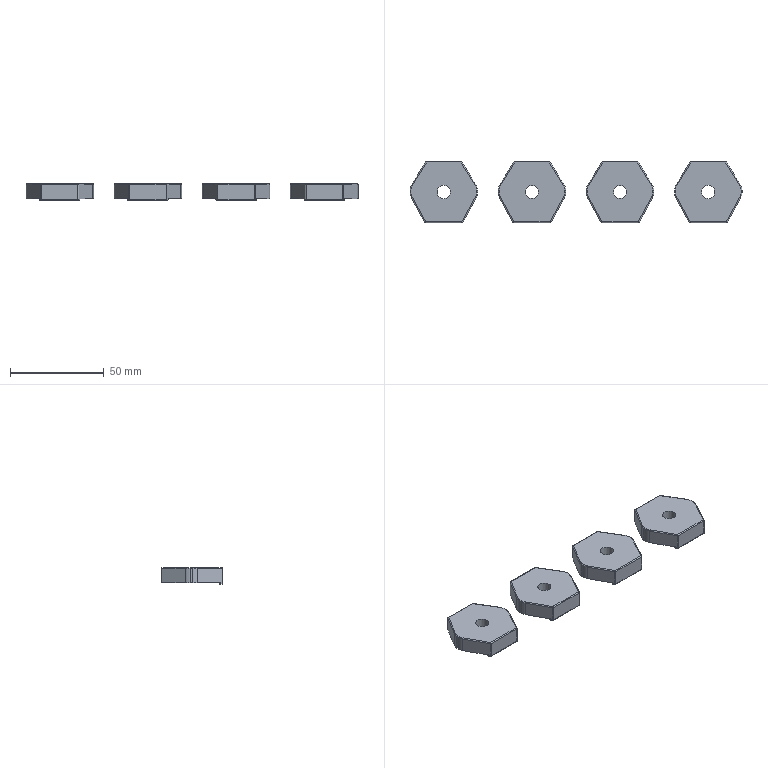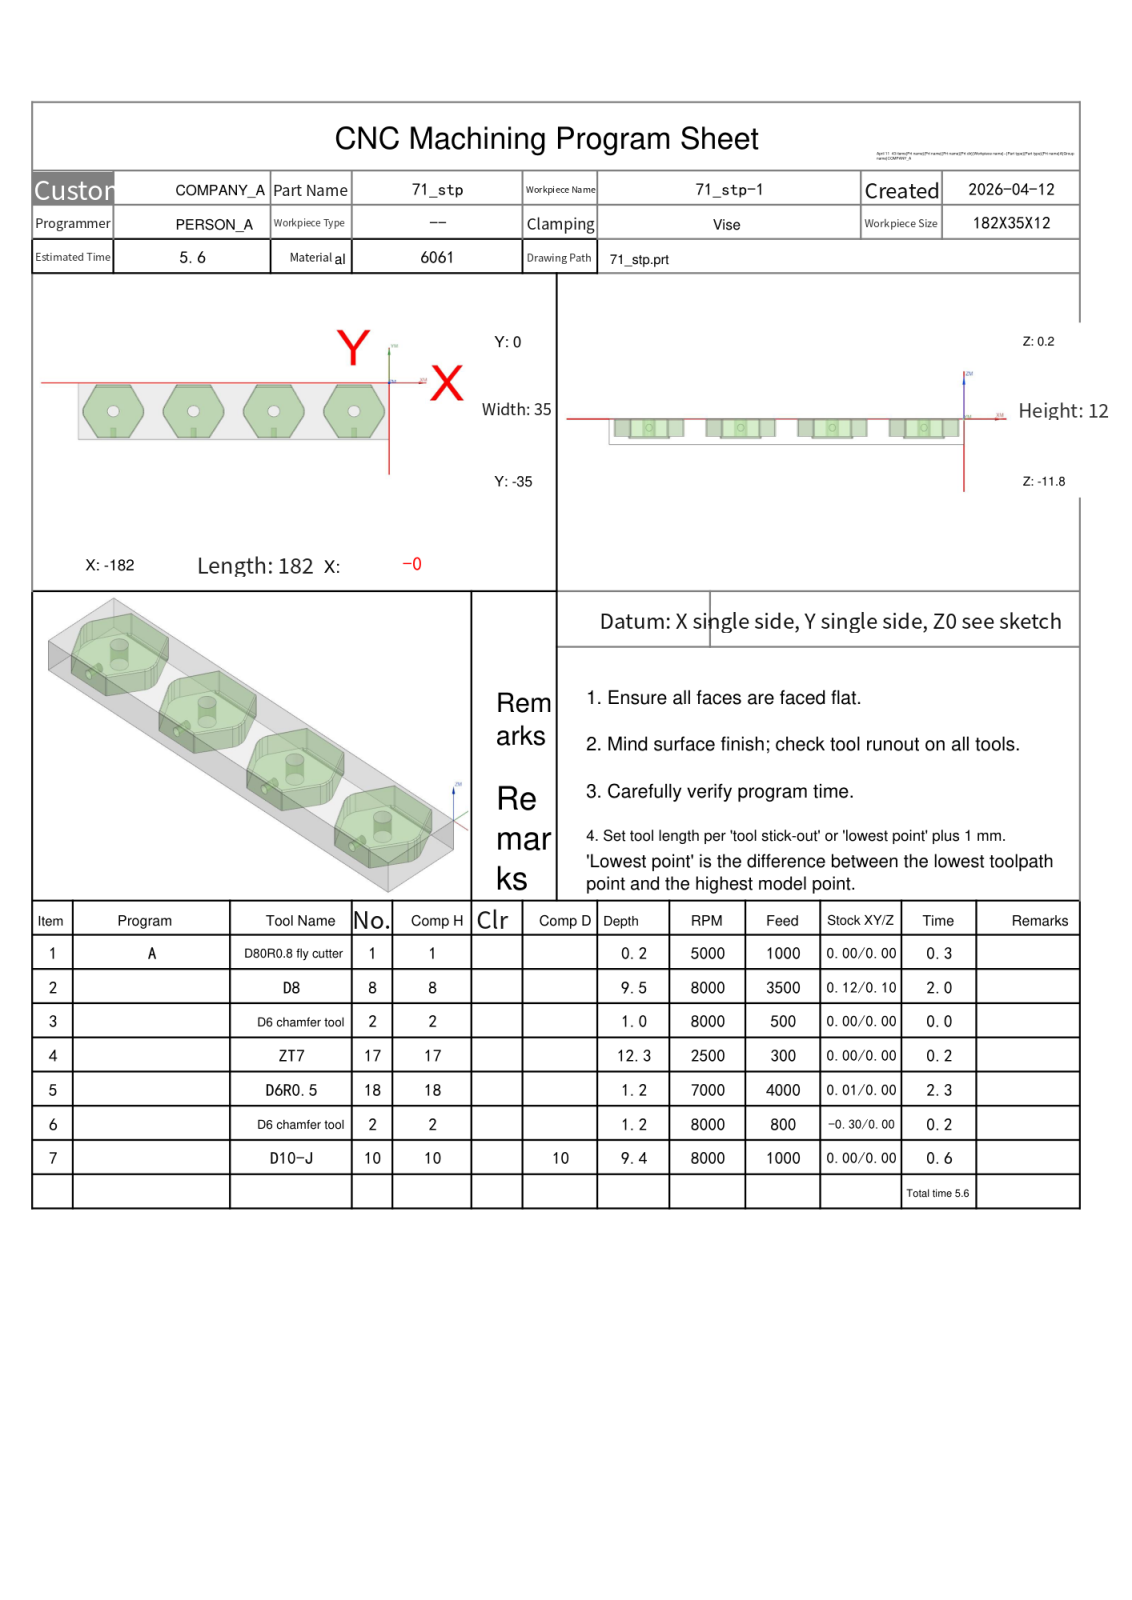NC program | NX | posted by the shop | part box 177 x 33 x 9 mm
Lines 3114 to 4443 of 15773:
N5 T18 M06
(D6R0.5  D=6. R=0.5 H=18 ce=0.01 di=0.00)
(MAX_Z=20. MIN_Z=-1. Time=2.28M)
G00 G90 G54 X-38.65 Y-23.77 M03 S7000
G43 H18 Z20.
M08
Z1.5
G01 X-39.759 Y-21.951 Z1.388 F4000.
X-40.062 Y-21.345 Z1.353
X-40.306 Y-20.712 Z1.317
X-40.489 Y-20.059 Z1.282
X-40.61 Y-19.392 Z1.246
X-40.668 Y-18.716 Z1.211
Y-16.764 Z1.108
X-40.599 Y-16.011 Z1.069
X-40.453 Y-15.269 Z1.029
X-40.228 Y-14.547 Z.989
X-39.929 Y-13.852 Z.95
X-32.47 Y-.086 Z.129
X-32.218 Y.255 Z.107
X-31.915 Y.551 Z.085
X-31.57 Y.796 Z.063
X-31.19 Y.983 Z.04
X-30.785 Y1.108 Z.018
X-30.366 Y1.168 Z-.004
X-30.202 Z-.012
X-10.798
G02 X-8.452 Y-.229 I0.0 J-2.668
G01 X-1.198 Y-13.617
G02 X-.332 Y-17.032 I-6.302 J-3.415
G01 Y-18.448
G02 X-1.38 Y-22.18 I-7.168 J0.0
G01 X-9.13 Y-34.889
G02 X-11.408 Y-36.168 I-2.277 J1.389
G01 X-29.592
G02 X-31.87 Y-34.889 I0.0 J2.668
G01 X-39.62 Y-22.18
G02 X-40.668 Y-18.448 I6.12 J3.732
G01 Y-17.032
G02 X-39.802 Y-13.617 I7.168 J0.0
G01 X-32.548 Y-.229
G02 X-30.202 Y1.168 I2.345 J-1.271
G01 X-27.777 Y1.169 Z-.013
X-25.351 Y1.172
X-22.926 Y1.175 Z-.014
X-20.5 Y1.177
X-18.074 Y1.18 Z-.015
X-15.649 Y1.182
X-13.223 Y1.184
X-10.798 Y1.187 Z-.016
X-10.637 Y1.182
X-10.478 Y1.168
X-10.319 Y1.144
X-10.162 Y1.111
X-10.008 Y1.069
X-9.856 Y1.017
X-9.707 Y.957
X-9.563 Y.887
X-9.422 Y.81
X-9.287 Y.724
X-9.157 Y.63
X-9.033 Y.528
X-8.915 Y.419
X-8.804 Y.304
X-8.699 Y.182
X-8.603 Y.054
X-8.514 Y-.08
X-8.433 Y-.219
X-7.222 Y-2.449 Z-.017
X-6.011 Y-4.679
X-4.799 Y-6.909 Z-.018
X-3.589 Y-9.14
X-2.377 Y-11.369 Z-.019
X-1.167 Y-13.6
X-1.106 Y-13.713
X-1.049 Y-13.826
X-.993 Y-13.941
X-.939 Y-14.057
X-.887 Y-14.174
X-.837 Y-14.292
X-.79 Y-14.41
X-.745 Y-14.53
X-.701 Y-14.65
X-.659 Y-14.771
X-.62 Y-14.892
X-.584 Y-15.015
X-.548 Y-15.137
X-.516 Y-15.261
X-.485 Y-15.385
X-.458 Y-15.51
X-.431 Y-15.635
X-.407 Y-15.76
X-.386 Y-15.886
X-.367 Y-16.013
X-.35 Y-16.139
X-.335 Y-16.266
X-.322 Y-16.393
X-.312 Y-16.521 Z-.02
X-.298 Y-16.776
X-.294 Y-17.032
X-.292 Y-17.74
X-.293 Y-18.448
X-.296 Y-18.695
X-.309 Y-18.941
X-.329 Y-19.187
X-.359 Y-19.432
X-.396 Y-19.676
X-.443 Y-19.918
X-.497 Y-20.159
X-.559 Y-20.398
X-.63 Y-20.634
X-.708 Y-20.868
X-.795 Y-21.099
X-.889 Y-21.327
X-.991 Y-21.552
X-1.101 Y-21.773
X-1.218 Y-21.99
X-1.343 Y-22.203 Z-.021
X-2.633 Y-24.322
X-3.923 Y-26.441
X-5.213 Y-28.561 Z-.022
X-6.502 Y-30.68
X-7.793 Y-32.798 Z-.023
X-9.082 Y-34.918
X-9.167 Y-35.048
X-9.258 Y-35.173
X-9.356 Y-35.292
X-9.462 Y-35.406
X-9.573 Y-35.513
X-9.69 Y-35.614
X-9.813 Y-35.709
X-9.941 Y-35.796
X-10.074 Y-35.876
X-10.211 Y-35.948
X-10.352 Y-36.012
X-10.496 Y-36.068
X-10.643 Y-36.116
X-10.793 Y-36.155
X-10.945 Y-36.186 Z-.024
X-11.098 Y-36.208
X-11.253 Y-36.221
X-11.408 Y-36.225
X-13.681 Y-36.226
X-15.954 Y-36.229
X-18.227 Y-36.23 Z-.025
X-20.5 Y-36.232
X-22.773 Y-36.234 Z-.026
X-25.046 Y-36.236
X-27.319 Y-36.237
X-29.592 Y-36.239 Z-.027
X-29.748 Y-36.235
X-29.903 Y-36.221
X-30.057 Y-36.2
X-30.21 Y-36.169
X-30.361 Y-36.13
X-30.509 Y-36.082
X-30.654 Y-36.026
X-30.796 Y-35.961
X-30.934 Y-35.889
X-31.067 Y-35.809
X-31.197 Y-35.722
X-31.32 Y-35.627
X-31.438 Y-35.526
X-31.55 Y-35.418
X-31.657 Y-35.303
X-31.755 Y-35.183
X-31.848 Y-35.058
X-31.933 Y-34.927
X-33.226 Y-32.81 Z-.028
X-34.519 Y-30.693
X-35.813 Y-28.576 Z-.029
X-37.105 Y-26.458
X-38.399 Y-24.341
X-39.692 Y-22.224 Z-.03
X-39.817 Y-22.01
X-39.936 Y-21.792
X-40.046 Y-21.57
X-40.15 Y-21.344
X-40.245 Y-21.115
X-40.332 Y-20.883
X-40.412 Y-20.647
X-40.483 Y-20.41
X-40.546 Y-20.17
X-40.601 Y-19.928
X-40.648 Y-19.684
X-40.686 Y-19.438
X-40.716 Y-19.192
X-40.738 Y-18.945
X-40.75 Y-18.697
X-40.755 Y-18.448
X-40.756 Y-17.74 Z-.031
Y-17.032
X-40.751 Y-16.774
X-40.738 Y-16.517
X-40.715 Y-16.261
X-40.684 Y-16.006
X-40.643 Y-15.751
X-40.593 Y-15.499
X-40.534 Y-15.248
X-40.467 Y-15.
X-40.391 Y-14.754
X-40.306 Y-14.511
X-40.212 Y-14.271
X-40.11 Y-14.035
X-40. Y-13.802
X-39.882 Y-13.574
X-38.674 Y-11.342 Z-.032
X-37.466 Y-9.11
X-36.259 Y-6.877 Z-.033
X-35.051 Y-4.645
X-33.843 Y-2.414 Z-.034
X-32.636 Y-.181
X-32.596 Y-.109
X-32.553 Y-.038
X-32.509 Y.031
X-32.462 Y.099
X-32.413 Y.166
X-32.363 Y.231
X-32.31 Y.295
X-32.255 Y.357
X-32.199 Y.418
X-32.141 Y.476
X-32.081 Y.533
X-32.02 Y.588
X-31.957 Y.642
X-31.892 Y.693
X-31.826 Y.743
X-31.758 Y.79
X-31.689 Y.836
X-31.619 Y.879
X-31.548 Y.92
X-31.475 Y.959
X-31.401 Y.997
X-31.326 Y1.031
X-31.25 Y1.064
X-31.173 Y1.093
X-31.095 Y1.122
X-31.016 Y1.147
X-30.937 Y1.17
X-30.857 Y1.191
X-30.777 Y1.21
X-30.695 Y1.225
X-30.614 Y1.239
X-30.532 Y1.25
X-30.367 Y1.265
X-30.202 Y1.27 Z-.035
X-27.777 Y1.272
X-25.351 Y1.274 Z-.036
X-22.926 Y1.276
X-20.5 Y1.279 Z-.037
X-18.074 Y1.28 Z-.038
X-15.649 Y1.283
X-13.223 Y1.285 Z-.039
X-10.798 Y1.287
X-10.715 Y1.286
X-10.632 Y1.283
X-10.549 Y1.277
X-10.466 Y1.268
X-10.383 Y1.257
X-10.301 Y1.243
X-10.22 Y1.227
X-10.139 Y1.209
X-10.058 Y1.188 Z-.04
X-9.978 Y1.165
X-9.899 Y1.139
X-9.821 Y1.111
X-9.743 Y1.081
X-9.667 Y1.049
X-9.591 Y1.014
X-9.516 Y.977
X-9.443 Y.938
X-9.371 Y.896
X-9.3 Y.853
X-9.231 Y.807
X-9.162 Y.759
X-9.096 Y.709
X-9.03 Y.658
X-8.967 Y.604
X-8.905 Y.549
X-8.845 Y.491
X-8.786 Y.432
X-8.729 Y.371
X-8.674 Y.309
X-8.621 Y.244
X-8.57 Y.179
X-8.521 Y.112
X-8.473 Y.043
X-8.429 Y-.027
X-8.385 Y-.098
X-8.345 Y-.171
X-7.134 Y-2.401 Z-.041
X-5.923 Y-4.632
X-4.712 Y-6.862 Z-.042
X-3.501 Y-9.092 Z-.043
X-2.29 Y-11.322
X-1.08 Y-13.553 Z-.044
X-.96 Y-13.782
X-.849 Y-14.016
X-.746 Y-14.254
X-.652 Y-14.495
X-.565 Y-14.74
X-.489 Y-14.987
X-.42 Y-15.237
X-.361 Y-15.489
X-.31 Y-15.743
X-.269 Y-15.999
X-.236 Y-16.256 Z-.045
X-.214 Y-16.514
X-.199 Y-16.773
X-.194 Y-17.032
Y-17.74
Y-18.448
X-.197 Y-18.699
X-.21 Y-18.948
X-.231 Y-19.197
X-.261 Y-19.446
X-.299 Y-19.693
X-.346 Y-19.939
X-.401 Y-20.183 Z-.046
X-.464 Y-20.424
X-.535 Y-20.664
X-.615 Y-20.901
X-.703 Y-21.135
X-.799 Y-21.366
X-.902 Y-21.594
X-1.014 Y-21.818
X-1.133 Y-22.038
X-1.259 Y-22.254
X-2.549 Y-24.373 Z-.047
X-3.839 Y-26.492
X-5.129 Y-28.612 Z-.048
X-6.419 Y-30.731 Z-.049
X-7.709 Y-32.85
X-8.999 Y-34.969 Z-.05
X-9.086 Y-35.103
X-9.181 Y-35.233
X-9.283 Y-35.357
X-9.391 Y-35.474
X-9.507 Y-35.586
X-9.628 Y-35.691
X-9.756 Y-35.788
X-9.888 Y-35.879
X-10.026 Y-35.961
X-10.168 Y-36.036
X-10.314 Y-36.102
X-10.463 Y-36.16
X-10.616 Y-36.21
X-10.771 Y-36.25
X-10.928 Y-36.282
X-11.087 Y-36.305
X-11.247 Y-36.319
X-11.408 Y-36.323
X-13.681 Y-36.325 Z-.051
X-15.954 Y-36.327 Z-.052
X-18.227 Y-36.328
X-20.5 Y-36.33 Z-.053
X-22.773 Y-36.331
X-25.046 Y-36.333 Z-.054
X-27.319 Y-36.335
X-29.592 Y-36.337 Z-.055
X-29.754 Y-36.332
X-29.914 Y-36.318
X-30.074 Y-36.296
X-30.232 Y-36.264
X-30.388 Y-36.224
X-30.542 Y-36.174
X-30.692 Y-36.116
X-30.839 Y-36.049
X-30.982 Y-35.974
X-31.12 Y-35.891
X-31.254 Y-35.801
X-31.382 Y-35.703
X-31.504 Y-35.598 Z-.056
X-31.62 Y-35.486
X-31.73 Y-35.368
X-31.833 Y-35.243
X-31.928 Y-35.113
X-32.016 Y-34.978
X-33.309 Y-32.861
X-34.602 Y-30.743 Z-.057
X-35.895 Y-28.626 Z-.058
X-37.188 Y-26.509
X-38.481 Y-24.392 Z-.059
X-39.775 Y-22.275
X-39.902 Y-22.058
X-40.022 Y-21.837 Z-.06
X-40.134 Y-21.612
X-40.239 Y-21.383
X-40.336 Y-21.151
X-40.424 Y-20.915
X-40.505 Y-20.677
X-40.577 Y-20.436
X-40.641 Y-20.193
X-40.697 Y-19.947
X-40.744 Y-19.7
X-40.783 Y-19.452
X-40.813 Y-19.202
X-40.835 Y-18.951
X-40.848 Y-18.7
X-40.852 Y-18.448
Y-17.74 Z-.061
X-40.853 Y-17.032
X-40.849 Y-16.771
X-40.835 Y-16.51
X-40.812 Y-16.251
X-40.78 Y-15.992
X-40.739 Y-15.734
X-40.688 Y-15.478
X-40.629 Y-15.224
X-40.561 Y-14.973
X-40.483 Y-14.723
X-40.397 Y-14.477
X-40.302 Y-14.234
X-40.199 Y-13.995 Z-.062
X-40.087 Y-13.759
X-39.967 Y-13.527
X-38.76 Y-11.295
X-37.552 Y-9.063 Z-.063
X-36.345 Y-6.831 Z-.064
X-35.137 Y-4.599
X-33.929 Y-2.367 Z-.065
X-32.722 Y-.135
X-32.68 Y-.06
X-32.636 Y.013 Z-.066
X-32.59 Y.085
X-32.541 Y.156
X-32.491 Y.225
X-32.438 Y.292
X-32.384 Y.358
X-32.328 Y.422
X-32.27 Y.485
X-32.209 Y.546
X-32.148 Y.605
X-32.084 Y.662
X-32.019 Y.717
X-31.952 Y.77
X-31.883 Y.822
X-31.813 Y.871
X-31.742 Y.918
X-31.669 Y.963
X-31.595 Y1.006
X-31.519 Y1.046
X-31.443 Y1.085
X-31.365 Y1.12
X-31.287 Y1.154
X-31.207 Y1.185
X-31.127 Y1.214
X-31.045 Y1.24
X-30.963 Y1.264
X-30.88 Y1.286
X-30.797 Y1.305
X-30.713 Y1.321
X-30.628 Y1.336
X-30.544 Y1.347
X-30.459 Y1.356
X-30.373 Y1.362
X-30.288 Y1.366
X-30.202 Y1.368
X-27.777 Y1.369 Z-.067
X-25.351 Y1.372 Z-.068
X-22.926 Y1.373 Z-.069
X-20.5 Y1.376
X-18.074 Y1.377 Z-.07
X-15.649 Y1.38 Z-.071
X-13.223 Y1.381 Z-.072
X-10.798 Y1.383
X-10.643 Y1.379
X-10.489 Y1.367 Z-.073
X-10.335 Y1.346
X-10.183 Y1.318
X-10.033 Y1.281
X-9.884 Y1.236
X-9.739 Y1.183
X-9.596 Y1.122
X-9.457 Y1.054
X-9.322 Y.978
X-9.191 Y.896
X-9.064 Y.806
X-8.943 Y.71
X-8.827 Y.607
X-8.717 Y.498
X-8.612 Y.384
X-8.514 Y.264
X-8.423 Y.139
X-8.338 Y.009
X-8.261 Y-.125
X-7.05 Y-2.356 Z-.074
X-5.839 Y-4.586 Z-.075
X-4.629 Y-6.817 Z-.076
X-3.418 Y-9.047 Z-.077
X-2.207 Y-11.277
X-.996 Y-13.507 Z-.078
X-.875 Y-13.74
X-.762 Y-13.977
X-.658 Y-14.218 Z-.079
X-.562 Y-14.462
X-.475 Y-14.71
X-.397 Y-14.96
X-.328 Y-15.213
X-.268 Y-15.469
X-.217 Y-15.726
X-.175 Y-15.985
X-.142 Y-16.246
X-.119 Y-16.507
X-.104 Y-16.769
X-.1 Y-17.032
X-.099 Y-17.74 Z-.08
Y-18.448
X-.103 Y-18.702
X-.116 Y-18.955
X-.137 Y-19.207
X-.167 Y-19.459
X-.206 Y-19.709
X-.253 Y-19.958
X-.309 Y-20.205
X-.373 Y-20.45 Z-.081
X-.445 Y-20.693
X-.526 Y-20.933
X-.615 Y-21.17
X-.712 Y-21.404
X-.817 Y-21.635
X-.93 Y-21.862
X-1.05 Y-22.085
X-1.178 Y-22.303
X-2.469 Y-24.422 Z-.082
X-3.758 Y-26.542 Z-.083
X-5.049 Y-28.66 Z-.084
X-6.338 Y-30.78
X-7.629 Y-32.899 Z-.085
X-8.918 Y-35.018 Z-.086
X-9.009 Y-35.157
X-9.106 Y-35.291
X-9.212 Y-35.418
X-9.324 Y-35.54
X-9.444 Y-35.655
X-9.569 Y-35.764
X-9.701 Y-35.864
X-9.838 Y-35.958
X-9.98 Y-36.043
X-10.126 Y-36.12
X-10.277 Y-36.189 Z-.087
X-10.432 Y-36.249
X-10.59 Y-36.3
X-10.75 Y-36.342
X-10.912 Y-36.375
X-11.077 Y-36.399
X-11.242 Y-36.413
X-11.408 Y-36.418
X-13.681 Y-36.419 Z-.088
X-15.954 Y-36.421
X-18.227 Y-36.422 Z-.089
X-20.5 Y-36.424 Z-.09
X-22.773 Y-36.426 Z-.091
X-25.046 Y-36.427
X-27.319 Y-36.429 Z-.092
X-29.592 Y-36.43 Z-.093
X-29.759 Y-36.426
X-29.925 Y-36.411
X-30.09 Y-36.388
X-30.253 Y-36.355
X-30.414 Y-36.313
X-30.573 Y-36.262
X-30.728 Y-36.202
X-30.88 Y-36.133
X-31.028 Y-36.056
X-31.17 Y-35.97
X-31.308 Y-35.877
X-31.441 Y-35.775
X-31.567 Y-35.667
X-31.687 Y-35.551
X-31.8 Y-35.429 Z-.094
X-31.906 Y-35.301
X-32.005 Y-35.166
X-32.096 Y-35.027
X-33.389 Y-32.909
X-34.682 Y-30.792 Z-.095
X-35.975 Y-28.675 Z-.096
X-37.268 Y-26.558 Z-.097
X-38.561 Y-24.44 Z-.098
X-39.854 Y-22.323
X-39.983 Y-22.104 Z-.099
X-40.105 Y-21.88
X-40.218 Y-21.652
X-40.324 Y-21.42
X-40.422 Y-21.185
X-40.512 Y-20.946
X-40.593 Y-20.705
X-40.666 Y-20.461
X-40.731 Y-20.215
X-40.788 Y-19.966
X-40.836 Y-19.716
X-40.875 Y-19.464
X-40.905 Y-19.212
X-40.927 Y-18.958 Z-.1
X-40.941 Y-18.703
X-40.945 Y-18.448
X-40.946 Y-17.74
Y-17.032
X-40.942 Y-16.768
X-40.928 Y-16.504
X-40.904 Y-16.241
X-40.872 Y-15.979 Z-.101
X-40.83 Y-15.718
X-40.779 Y-15.459
X-40.719 Y-15.201
X-40.65 Y-14.947
X-40.571 Y-14.694
X-40.484 Y-14.445
X-40.388 Y-14.199
X-40.284 Y-13.956
X-40.17 Y-13.718
X-40.049 Y-13.483
X-38.841 Y-11.251 Z-.102
X-37.634 Y-9.019 Z-.103
X-36.426 Y-6.787 Z-.104
X-35.219 Y-4.555 Z-.105
X-34.011 Y-2.323
X-32.803 Y-.091 Z-.106
X-32.724 Y.047
X-32.637 Y.18
X-32.544 Y.309
X-32.443 Y.432
X-32.336 Y.549
X-32.223 Y.661 Z-.107
X-32.105 Y.767
X-31.98 Y.865
X-31.851 Y.958
X-31.716 Y1.043
X-31.578 Y1.12
X-31.435 Y1.19
X-31.289 Y1.253
X-31.14 Y1.307
X-30.988 Y1.354
X-30.833 Y1.392
X-30.677 Y1.422
X-30.52 Y1.443
X-30.361 Y1.456
X-30.202 Y1.461
X-27.777 Y1.462 Z-.108
X-25.351 Y1.464 Z-.109
X-22.926 Y1.465 Z-.11
X-20.5 Y1.468 Z-.111
X-18.074 Y1.469 Z-.112
X-15.649 Y1.471 Z-.113
X-13.223 Y1.473 Z-.114
X-10.798 Y1.475 Z-.115
X-10.638 Y1.471
X-10.479 Y1.458
X-10.32 Y1.437
X-10.163 Y1.407
X-10.008 Y1.369
X-9.855 Y1.322
X-9.705 Y1.268
X-9.558 Y1.205
X-9.415 Y1.135
X-9.275 Y1.057
X-9.14 Y.972
X-9.01 Y.879
X-8.884 Y.78 Z-.116
X-8.765 Y.674
X-8.651 Y.562
X-8.543 Y.443
X-8.442 Y.32
X-8.348 Y.191
X-8.26 Y.057
X-8.18 Y-.082
X-6.97 Y-2.312 Z-.117
X-5.759 Y-4.543 Z-.118
X-4.548 Y-6.773 Z-.119
X-3.338 Y-9.003 Z-.12
X-2.127 Y-11.234 Z-.121
X-.916 Y-13.464 Z-.122
X-.794 Y-13.7
X-.68 Y-13.94
X-.574 Y-14.183
X-.477 Y-14.431
X-.389 Y-14.681
X-.31 Y-14.935 Z-.123
X-.24 Y-15.191
X-.179 Y-15.45
X-.128 Y-15.71
X-.085 Y-15.973
X-.052 Y-16.236
X-.029 Y-16.501
X-.014 Y-16.766
X-.009 Y-17.032
Y-17.74 Z-.124
X-.008 Y-18.448
X-.012 Y-18.705
X-.025 Y-18.961
X-.047 Y-19.216
X-.078 Y-19.471
X-.117 Y-19.724
X-.165 Y-19.976
X-.221 Y-20.227 Z-.125
X-.286 Y-20.475
X-.359 Y-20.72
X-.441 Y-20.963
X-.531 Y-21.204
X-.629 Y-21.44
X-.735 Y-21.674
X-.85 Y-21.903
X-.971 Y-22.129
X-1.101 Y-22.351
X-2.391 Y-24.469 Z-.126
X-3.681 Y-26.588 Z-.127
X-4.972 Y-28.707 Z-.128
X-6.262 Y-30.827 Z-.129
X-7.552 Y-32.945 Z-.13
X-8.842 Y-35.065 Z-.131
X-8.935 Y-35.208
X-9.036 Y-35.346
X-9.144 Y-35.477
X-9.26 Y-35.603
X-9.383 Y-35.722 Z-.132
X-9.512 Y-35.833
X-9.648 Y-35.937
X-9.789 Y-36.033
X-9.936 Y-36.121
X-10.087 Y-36.201
X-10.243 Y-36.271
X-10.402 Y-36.333
X-10.564 Y-36.386
X-10.73 Y-36.429
X-10.897 Y-36.463
X-11.066 Y-36.488
X-11.237 Y-36.502
X-11.408 Y-36.507
X-13.681 Y-36.508 Z-.133
X-15.954 Y-36.51 Z-.134
X-18.227 Y-36.511 Z-.135
X-20.5 Y-36.513 Z-.136
X-22.773 Y-36.514 Z-.137
X-25.046 Y-36.516 Z-.138
X-27.319 Y-36.518 Z-.139
X-29.592 Y-36.519
X-29.678 Y-36.518
X-29.764 Y-36.514 Z-.14
X-29.85 Y-36.508
X-29.935 Y-36.5
X-30.02 Y-36.489
X-30.105 Y-36.476
X-30.189 Y-36.46
X-30.273 Y-36.442
X-30.357 Y-36.421
X-30.439 Y-36.399
X-30.521 Y-36.373
X-30.603 Y-36.346
X-30.683 Y-36.316
X-30.763 Y-36.284
X-30.841 Y-36.25
X-30.919 Y-36.213
X-30.996 Y-36.174
X-31.071 Y-36.133
X-31.145 Y-36.09
X-31.218 Y-36.045
X-31.29 Y-35.998
X-31.36 Y-35.949
X-31.429 Y-35.898
X-31.497 Y-35.844
X-31.563 Y-35.79
X-31.627 Y-35.733
X-31.69 Y-35.674
X-31.75 Y-35.613
X-31.81 Y-35.551
X-31.867 Y-35.488
X-31.923 Y-35.422
X-31.976 Y-35.355 Z-.141
X-32.028 Y-35.287
X-32.078 Y-35.217
X-32.126 Y-35.146
X-32.172 Y-35.073
X-33.465 Y-32.955 Z-.142
X-34.758 Y-30.838 Z-.143
X-36.05 Y-28.721 Z-.144
X-37.344 Y-26.604
X-38.636 Y-24.486 Z-.145
X-39.93 Y-22.369 Z-.146
X-40.06 Y-22.147 Z-.147
X-40.183 Y-21.92
X-40.298 Y-21.69
X-40.405 Y-21.455
X-40.504 Y-21.217
X-40.595 Y-20.976
X-40.677 Y-20.732
X-40.751 Y-20.485
X-40.817 Y-20.236
X-40.874 Y-19.984
X-40.923 Y-19.731 Z-.148
X-40.962 Y-19.476
X-40.993 Y-19.221
X-41.015 Y-18.964
X-41.029 Y-18.706
X-41.033 Y-18.448
X-41.034 Y-17.74
Y-17.032 Z-.149
X-41.03 Y-16.764
X-41.016 Y-16.498
X-40.992 Y-16.231
X-40.959 Y-15.966
X-40.917 Y-15.702
X-40.865 Y-15.44
X-40.804 Y-15.18
X-40.734 Y-14.922
X-40.655 Y-14.667
X-40.567 Y-14.414 Z-.15
X-40.47 Y-14.165
X-40.364 Y-13.92
X-40.249 Y-13.678
X-40.126 Y-13.441
X-38.919 Y-11.209 Z-.151
X-37.711 Y-8.977 Z-.152
X-36.503 Y-6.745 Z-.153
X-35.296 Y-4.513 Z-.154
X-34.088 Y-2.281 Z-.155
X-32.88 Y-.049 Z-.156
X-32.799 Y.093
X-32.709 Y.23
X-32.613 Y.362
X-32.51 Y.489
X-32.4 Y.61
X-32.283 Y.725
X-32.161 Y.834
X-32.033 Y.935
X-31.899 Y1.03
X-31.761 Y1.118 Z-.157
X-31.618 Y1.198
X-31.472 Y1.27
X-31.321 Y1.334
X-31.167 Y1.39
X-31.011 Y1.438
X-30.852 Y1.477
X-30.691 Y1.508
X-30.529 Y1.53
X-30.366 Y1.543
X-30.202 Y1.548
X-27.777 Y1.549 Z-.158
X-25.351 Y1.551 Z-.159
X-22.926 Y1.553 Z-.16
X-20.5 Y1.555 Z-.162
X-18.074 Y1.556 Z-.163
X-15.649 Y1.558 Z-.164
X-13.223 Y1.56 Z-.165
X-10.798 Y1.561 Z-.166
X-10.633 Y1.557
X-10.47 Y1.544
X-10.307 Y1.522
X-10.145 Y1.491
X-9.985 Y1.452
X-9.828 Y1.404
X-9.673 Y1.348
X-9.522 Y1.284
X-9.374 Y1.211 Z-.167
X-9.231 Y1.131
X-9.092 Y1.043
X-8.958 Y.948
X-8.829 Y.846
X-8.706 Y.737
X-8.588 Y.622
X-8.478 Y.5
X-8.373 Y.373
X-8.276 Y.24
X-8.187 Y.102
X-8.104 Y-.041
X-6.894 Y-2.271 Z-.169
X-5.683 Y-4.501 Z-.17
X-4.473 Y-6.732 Z-.171
X-3.262 Y-8.962 Z-.172
X-2.052 Y-11.193 Z-.173
X-.841 Y-13.423 Z-.174
X-.717 Y-13.662
X-.602 Y-13.904
X-.495 Y-14.151 Z-.175
X-.397 Y-14.401
X-.308 Y-14.654
X-.228 Y-14.911
X-.157 Y-15.17
X-.096 Y-15.432
X-.043 Y-15.695
X-.001 Y-15.96
X.033 Y-16.227 Z-.176
X.057 Y-16.495
X.071 Y-16.763
X.076 Y-17.032
X.077 Y-17.74
Y-18.448 Z-.177
X.073 Y-18.708
X.06 Y-18.967
X.038 Y-19.225
X.007 Y-19.482
X-.033 Y-19.739
X-.081 Y-19.994
X-.138 Y-20.247
X-.204 Y-20.497
X-.278 Y-20.746 Z-.178
X-.361 Y-20.992
X-.452 Y-21.235
X-.551 Y-21.474
X-.658 Y-21.71
X-.774 Y-21.943
X-.897 Y-22.171
X-1.028 Y-22.395
X-2.319 Y-24.514 Z-.18
X-3.609 Y-26.633 Z-.181
X-4.899 Y-28.751 Z-.182
X-6.189 Y-30.871 Z-.183
X-7.48 Y-32.989 Z-.184
X-8.77 Y-35.109 Z-.185
X-8.816 Y-35.183
X-8.865 Y-35.256
X-8.916 Y-35.327
X-8.969 Y-35.398
X-9.024 Y-35.466
X-9.081 Y-35.533
X-9.139 Y-35.598
X-9.2 Y-35.662
X-9.262 Y-35.724
X-9.326 Y-35.784 Z-.186
X-9.392 Y-35.842
X-9.459 Y-35.899
X-9.528 Y-35.953
X-9.599 Y-36.006
X-9.671 Y-36.056
X-9.744 Y-36.104
X-9.819 Y-36.151
X-9.894 Y-36.195
X-9.972 Y-36.237
X-10.05 Y-36.277
X-10.129 Y-36.314
X-10.21 Y-36.349
X-10.291 Y-36.382
X-10.374 Y-36.413
X-10.457 Y-36.441
X-10.541 Y-36.467
X-10.625 Y-36.49
X-10.711 Y-36.512
X-10.797 Y-36.53
X-10.883 Y-36.546
X-10.97 Y-36.56
X-11.057 Y-36.571
X-11.144 Y-36.58
X-11.232 Y-36.586
X-11.32 Y-36.59 Z-.187
X-11.408 Y-36.592
X-13.681 Y-36.593 Z-.188
X-15.954 Y-36.594 Z-.189
X-18.227 Y-36.596 Z-.19
X-20.5 Y-36.597 Z-.191
X-22.773 Y-36.598 Z-.192
X-25.046 Y-36.6 Z-.193
X-27.319 Y-36.601 Z-.194
X-29.592 Y-36.603 Z-.195
X-29.681 Y-36.602
X-29.769 Y-36.598
X-29.857 Y-36.592
X-29.944 Y-36.583
X-30.032 Y-36.572
X-30.119 Y-36.558
X-30.206 Y-36.542
X-30.292 Y-36.523
X-30.378 Y-36.502
X-30.463 Y-36.479
X-30.547 Y-36.453
X-30.63 Y-36.424
X-30.713 Y-36.394
X-30.795 Y-36.361
X-30.876 Y-36.326
X-30.956 Y-36.288
X-31.034 Y-36.248
X-31.112 Y-36.206
X-31.188 Y-36.162 Z-.196
X-31.263 Y-36.116
X-31.337 Y-36.067
X-31.409 Y-36.016
X-31.48 Y-35.964
X-31.549 Y-35.909
X-31.617 Y-35.853
X-31.683 Y-35.794
X-31.748 Y-35.734
X-31.81 Y-35.672
X-31.871 Y-35.608
X-31.93 Y-35.542
X-31.987 Y-35.475
X-32.042 Y-35.406
X-32.096 Y-35.336
X-32.147 Y-35.264
X-32.196 Y-35.191
X-32.243 Y-35.116
X-33.536 Y-32.999 Z-.197
X-34.829 Y-30.882 Z-.198
X-36.122 Y-28.764 Z-.2
X-37.415 Y-26.647 Z-.201
X-38.707 Y-24.53 Z-.202
X-40.001 Y-22.412 Z-.203
X-40.132 Y-22.188
X-40.256 Y-21.959
X-40.373 Y-21.725
X-40.481 Y-21.488
X-40.581 Y-21.248
X-40.673 Y-21.004 Z-.204
X-40.756 Y-20.757
X-40.831 Y-20.507
X-40.898 Y-20.255
X-40.955 Y-20.001
X-41.004 Y-19.745
X-41.044 Y-19.488
X-41.076 Y-19.229
X-41.098 Y-18.969 Z-.205
X-41.111 Y-18.709
X-41.116 Y-18.448
Y-17.74
X-41.117 Y-17.032
X-41.112 Y-16.761 Z-.206
X-41.098 Y-16.492
X-41.074 Y-16.223
X-41.041 Y-15.954
X-40.998 Y-15.688
X-40.946 Y-15.423
X-40.884 Y-15.16
X-40.814 Y-14.899
X-40.733 Y-14.641
X-40.644 Y-14.386 Z-.207
X-40.546 Y-14.134
X-40.439 Y-13.886
X-40.323 Y-13.642
X-40.199 Y-13.402
X-38.991 Y-11.17 Z-.208
X-37.784 Y-8.938 Z-.209
X-36.575 Y-6.706 Z-.211
X-35.368 Y-4.474 Z-.212
X-34.16 Y-2.242 Z-.213
X-32.952 Y-.01 Z-.214
X-32.868 Y.136
X-32.777 Y.277
X-32.678 Y.412
X-32.572 Y.543
X-32.459 Y.667
X-32.339 Y.785
X-32.214 Y.896
X-32.082 Y1.001 Z-.215
X-31.945 Y1.098
X-31.803 Y1.188
X-31.657 Y1.27
X-31.506 Y1.345
X-31.351 Y1.411
X-31.193 Y1.468
X-31.033 Y1.517
X-30.869 Y1.558
X-30.704 Y1.589
X-30.538 Y1.612
X-30.37 Y1.625
X-30.202 Y1.63
X-27.777 Y1.631 Z-.217
X-25.351 Y1.633 Z-.218
X-22.926 Y1.634 Z-.219
X-20.5 Y1.636 Z-.22
X-18.074 Y1.637 Z-.222
X-15.649 Y1.639 Z-.223
X-13.223 Y1.64 Z-.224
X-10.798 Y1.642 Z-.225
X-10.629 Y1.638
X-10.461 Y1.624 Z-.226
X-10.294 Y1.602
X-10.128 Y1.57
X-9.964 Y1.53
X-9.802 Y1.481
X-9.644 Y1.423
X-9.488 Y1.357
X-9.337 Y1.283
X-9.19 Y1.2
X-9.047 Y1.11
X-8.909 Y1.013
X-8.777 Y.908
X-8.651 Y.796 Z-.227
X-8.53 Y.677
X-8.417 Y.553
X-8.31 Y.422
X-8.21 Y.286
X-8.118 Y.144
X-8.033 Y-.002
X-6.823 Y-2.232 Z-.228
X-5.613 Y-4.463 Z-.23
X-4.402 Y-6.694 Z-.231
X-3.192 Y-8.924 Z-.232
X-1.981 Y-11.155 Z-.234
X-.771 Y-13.385 Z-.235
X-.646 Y-13.626
X-.529 Y-13.871
X-.474 Y-13.995
X-.421 Y-14.12
X-.371 Y-14.246
X-.322 Y-14.373
X-.276 Y-14.501
X-.232 Y-14.629
X-.191 Y-14.759 Z-.236
X-.152 Y-14.889
X-.08 Y-15.15
X-.018 Y-15.415
X.035 Y-15.681
X.078 Y-15.949
X.112 Y-16.219
X.136 Y-16.489
X.151 Y-16.76 Z-.237
X.156 Y-17.032
Y-17.74
X.157 Y-18.448
X.152 Y-18.71 Z-.238
X.139 Y-18.972
X.117 Y-19.233
X.086 Y-19.493
X.046 Y-19.752
X-.003 Y-20.01
X-.061 Y-20.266
X-.127 Y-20.519 Z-.239
X-.202 Y-20.77
X-.286 Y-21.019
X-.378 Y-21.264
X-.478 Y-21.506
X-.587 Y-21.745
X-.704 Y-21.979
X-.828 Y-22.21
X-.961 Y-22.436 Z-.24
X-.97 Y-22.452
X-.98 Y-22.467
X-2.26 Y-24.571 Z-.241
X-3.541 Y-26.674 Z-.242
X-4.832 Y-28.793 Z-.243
X-6.122 Y-30.912 Z-.245
X-7.413 Y-33.03 Z-.246
X-8.703 Y-35.149 Z-.247
X-8.791 Y-35.286
X-8.885 Y-35.417
X-8.986 Y-35.544
X-9.094 Y-35.665
X-9.208 Y-35.78 Z-.248
X-9.327 Y-35.89
X-9.452 Y-35.993
X-9.582 Y-36.09
X-9.717 Y-36.18
X-9.856 Y-36.263
X-9.999 Y-36.339
X-10.146 Y-36.408
X-10.297 Y-36.468
X-10.45 Y-36.521
X-10.606 Y-36.566
X-10.763 Y-36.603
X-10.923 Y-36.632 Z-.249
X-11.084 Y-36.653
X-11.245 Y-36.666
X-11.408 Y-36.67
X-13.681 Y-36.671 Z-.25
X-15.954 Y-36.673 Z-.251
X-18.227 Y-36.674 Z-.252
X-20.5 Y-36.675 Z-.253
X-22.773 Y-36.676 Z-.255
X-25.046 Y-36.678 Z-.256
X-27.319 Y-36.679 Z-.257
X-29.592 Y-36.68 Z-.258
X-29.755 Y-36.676
X-29.917 Y-36.664
X-30.079 Y-36.643
X-30.239 Y-36.614
X-30.397 Y-36.577
X-30.554 Y-36.532 Z-.259
X-30.707 Y-36.479
X-30.858 Y-36.418
X-31.006 Y-36.35
X-31.15 Y-36.274
X-31.29 Y-36.191
X-31.425 Y-36.1
X-31.556 Y-36.003
X-31.681 Y-35.9
X-31.801 Y-35.79
X-31.916 Y-35.674
X-32.024 Y-35.552
X-32.126 Y-35.425 Z-.26
X-32.221 Y-35.293
X-32.309 Y-35.157
X-33.602 Y-33.039 Z-.261
X-34.895 Y-30.922 Z-.262
X-36.187 Y-28.804 Z-.264
X-37.48 Y-26.687 Z-.265
X-38.773 Y-24.57 Z-.266
X-40.066 Y-22.452 Z-.267
X-40.199 Y-22.225
X-40.324 Y-21.994 Z-.268
X-40.442 Y-21.758
X-40.551 Y-21.519
X-40.652 Y-21.276
X-40.745 Y-21.03
X-40.829 Y-20.78
X-40.905 Y-20.528
X-40.972 Y-20.274
X-41.03 Y-20.017 Z-.269
X-41.08 Y-19.758
X-41.12 Y-19.498
X-41.152 Y-19.237
X-41.174 Y-18.975
X-41.188 Y-18.712
X-41.192 Y-18.448
X-41.193 Y-17.74 Z-.27
Y-17.032
X-41.189 Y-16.759
X-41.174 Y-16.486
X-41.15 Y-16.214 Z-.271
X-41.117 Y-15.944
X-41.073 Y-15.674
X-41.021 Y-15.406
X-40.958 Y-15.141
X-40.887 Y-14.877
X-40.806 Y-14.617
X-40.716 Y-14.359 Z-.272
X-40.617 Y-14.105
X-40.509 Y-13.854
X-40.392 Y-13.608
X-40.266 Y-13.365
X-39.058 Y-11.133 Z-.273
X-37.85 Y-8.902 Z-.275
X-36.643 Y-6.67 Z-.276
X-35.435 Y-4.438 Z-.277
X-34.227 Y-2.206 Z-.279
X-33.019 Y.026 Z-.28
X-32.933 Y.175
X-32.839 Y.32
X-32.738 Y.459
X-32.629 Y.592
X-32.513 Y.719
X-32.391 Y.84
X-32.262 Y.954
X-32.128 Y1.062 Z-.281
X-31.987 Y1.161
X-31.842 Y1.253
X-31.692 Y1.337
X-31.537 Y1.413
X-31.379 Y1.481
X-31.217 Y1.54
X-31.053 Y1.59
X-30.886 Y1.631
X-30.716 Y1.664
X-30.546 Y1.687
X-30.374 Y1.701 Z-.282
X-30.202 Y1.706
X-27.777 Y1.707 Z-.283
X-25.351 Y1.708 Z-.284
X-22.926 Y1.71 Z-.286
X-20.5 Y1.711 Z-.287
X-18.074 Y1.713 Z-.288
X-15.649 Y1.714 Z-.29
X-13.223 Y1.715 Z-.291
X-10.798 Y1.716 Z-.292
X-10.625 Y1.712 Z-.293
X-10.453 Y1.698
X-10.282 Y1.675
X-10.112 Y1.643
X-9.944 Y1.602
X-9.779 Y1.551
X-9.616 Y1.492
X-9.458 Y1.425
X-9.302 Y1.349
X-9.152 Y1.264
X-9.005 Y1.172 Z-.294
X-8.865 Y1.072
X-8.729 Y.965
X-8.6 Y.85
X-8.477 Y.729
X-8.36 Y.601
X-8.251 Y.467
X-8.149 Y.328
X-8.055 Y.183
X-7.968 Y.033
X-6.758 Y-2.198 Z-.296
X-5.548 Y-4.428 Z-.297
X-4.338 Y-6.659 Z-.299
X-3.127 Y-8.889 Z-.3
X-1.917 Y-11.12 Z-.302
X-.706 Y-13.35 Z-.303
X-.58 Y-13.594
X-.462 Y-13.841
X-.353 Y-14.093
X-.254 Y-14.348 Z-.304
X-.163 Y-14.606
X-.081 Y-14.868
X-.009 Y-15.133
X.054 Y-15.399
X.107 Y-15.668
X.151 Y-15.939 Z-.305
X.185 Y-16.211
X.209 Y-16.484
X.224 Y-16.758
X.229 Y-17.032
X.23 Y-17.74 Z-.306
Y-18.448
X.225 Y-18.715
X.212 Y-18.982
X.189 Y-19.248
X.157 Y-19.512 Z-.307
X.116 Y-19.776
X.065 Y-20.038
X.006 Y-20.298
X-.062 Y-20.556
X-.139 Y-20.812
X-.225 Y-21.065
X-.319 Y-21.314 Z-.308
X-.422 Y-21.56
X-.534 Y-21.803
X-.654 Y-22.041
X-.773 Y-22.26
X-.899 Y-22.474
X-.908 Y-22.49
X-.917 Y-22.505
X-2.205 Y-24.618 Z-.31
X-3.492 Y-26.732 Z-.311
X-4.78 Y-28.846 Z-.313
X-6.067 Y-30.96 Z-.314
X-7.354 Y-33.073 Z-.315
X-8.641 Y-35.187 Z-.317
X-8.731 Y-35.326
X-8.828 Y-35.461
X-8.932 Y-35.59
X-9.042 Y-35.714
X-9.158 Y-35.832
X-9.28 Y-35.944
X-9.408 Y-36.05
X-9.541 Y-36.149
X-9.679 Y-36.241 Z-.318
X-9.821 Y-36.326
X-9.967 Y-36.403
X-10.118 Y-36.473
X-10.272 Y-36.535
X-10.428 Y-36.59